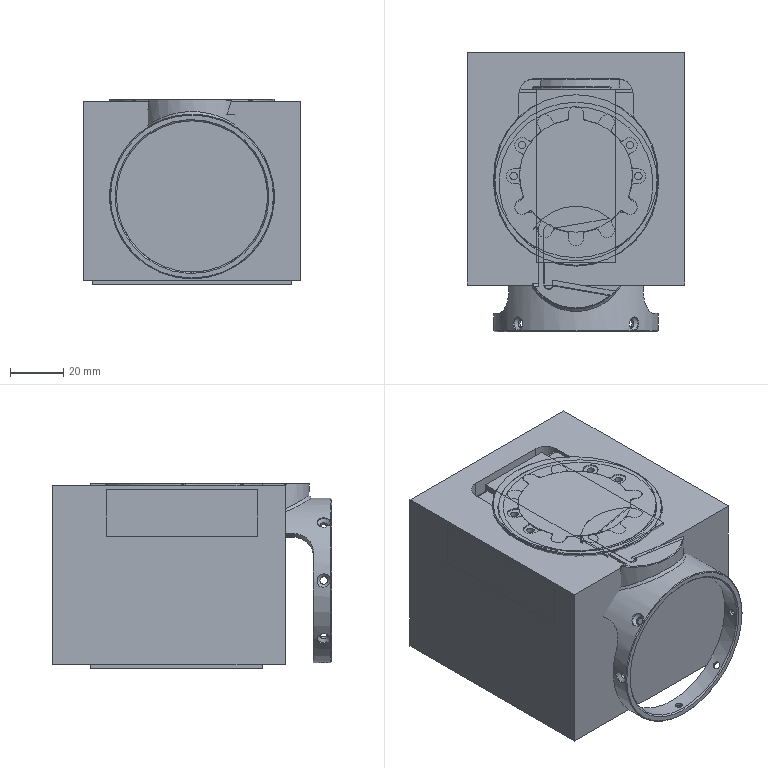NC program | NX | posted with a generic post | part box 82 x 105.2 x 70 mm
Lines 21226 to 22991 of 123648, first 1627 of 1738 lines:
(中心钻 , TOOL : 倒角刀D4)
N42414 T11 M6
N42416 G53
N42418 G19 G0 G90 Y31.15 Z-35. S2600 M3
N42420 G43 X-72.5 H11
N42422 G94 G81 G98 X-13.2 F200. R-15.
N42424 Y30.85 Z-31.5
N42426 Y31.15 Z-28.
N42428 Y30.85 Z-24.5
N42430 Y31.15 Z-21.
N42432 G80
(中心钻_COPY , TOOL : 倒角刀D4)
N42434 G17 G0 X-55. Y43.301
N42436 Z-28.
N42438 G81 X-23.135 Y16.562 F200. R-28.
N42440 G80
N42442 G0 X-53.52 Y45.117 Z-28.
N42444 X-51.98 Y46.883
N42446 X-50.382 Y48.597
N42448 X-48.727 Y50.256
N42450 X-47.018 Y51.859
N42452 X-45.256 Y53.403
N42454 X-43.443 Y54.888
N42456 X-41.582 Y56.311
N42458 X-39.673 Y57.672
N42460 X-37.721 Y58.967
N42462 X-35.726 Y60.197
N42464 X-33.691 Y61.359
N42466 X-31.619 Y62.452
N42468 X-29.511 Y63.475
N42470 X-27.37 Y64.427
N42472 X-25.198 Y65.307
N42474 X-22.998 Y66.114
N42476 X-20.772 Y66.847
N42478 X-18.523 Y67.505
N42480 X-16.254 Y68.087
N42482 X-13.966 Y68.593
N42484 X-11.662 Y69.022
N42486 X-9.345 Y69.373
N42488 X-7.018 Y69.647
N42490 X-4.683 Y69.843
N42492 X-2.343 Y69.961
N42494 G18 X0. Y70.
N42496 G17 X2.343 Y69.961
N42498 X4.683 Y69.843
N42500 X7.018 Y69.647
N42502 X9.345 Y69.373
N42504 X11.662 Y69.022
N42506 X13.966 Y68.593
N42508 X16.254 Y68.087
N42510 X18.523 Y67.505
N42512 X20.772 Y66.847
N42514 X22.998 Y66.114
N42516 X25.198 Y65.307
N42518 X27.37 Y64.427
N42520 X29.511 Y63.475
N42522 X31.619 Y62.452
N42524 X33.691 Y61.359
N42526 X35.726 Y60.197
N42528 X37.721 Y58.967
N42530 X39.673 Y57.672
N42532 X41.582 Y56.311
N42534 X43.443 Y54.888
N42536 X45.256 Y53.403
N42538 X47.018 Y51.859
N42540 X48.727 Y50.256
N42542 X50.382 Y48.597
N42544 X51.98 Y46.883
N42546 X53.52 Y45.117
N42548 X55. Y43.301
N42550 G81 X23.135 Y16.562 F200. R-28.
N42552 G80
(中心钻_COPY_COPY , TOOL : 倒角刀D4)
N42554 G0 Z-3.
N42556 X-50.902 Y48.052
N42558 G81 X-21.355 Y18.505 F200. R-3.
N42560 G80
N42562 G0 X-52.47 Y46.335 Z-3.
N42564 X-53.98 Y44.566
N42566 X-55.431 Y42.749
N42568 X-56.82 Y40.884
N42570 X-58.147 Y38.974
N42572 X-59.409 Y37.021
N42574 X-60.606 Y35.027
N42576 X-61.736 Y32.995
N42578 X-62.798 Y30.926
N42580 X-63.79 Y28.823
N42582 X-64.713 Y26.688
N42584 X-65.563 Y24.524
N42586 X-66.342 Y22.333
N42588 X-67.047 Y20.117
N42590 X-67.678 Y17.879
N42592 X-68.235 Y15.621
N42594 X-68.716 Y13.346
N42596 X-69.121 Y11.056
N42598 X-69.45 Y8.754
N42600 X-69.703 Y6.442
N42602 X-69.878 Y4.123
N42604 X-69.977 Y1.8
N42606 X-69.998 Y-0.525
N42608 G19 X-69.942 Y-2.85
N42610 G81 X-30.2 F200. R-32.
N42612 G80
N42614 G17 G0 X-69.807 Y-5.2 Z-3.
N42616 X-69.592 Y-7.544
N42618 X-69.299 Y-9.88
N42620 X-68.928 Y-12.204
N42622 X-68.479 Y-14.515
N42624 X-67.952 Y-16.809
N42626 X-67.348 Y-19.084
N42628 X-66.669 Y-21.338
N42630 X-65.913 Y-23.567
N42632 X-65.084 Y-25.77
N42634 X-64.18 Y-27.944
N42636 X-63.205 Y-30.086
N42638 X-62.157 Y-32.194
N42640 X-61.04 Y-34.266
N42642 X-59.853 Y-36.299
N42644 X-58.599 Y-38.291
N42646 X-57.278 Y-40.239
N42648 X-55.893 Y-42.142
N42650 X-54.444 Y-43.998
N42652 X-52.934 Y-45.804
N42654 X-51.364 Y-47.557
N42656 X-49.736 Y-49.258
N42658 X-48.052 Y-50.902
N42660 G81 X-21.355 Y-24.205 F200. R-3.
N42662 G80
N42664 G0 X-46.352 Y-52.455 Z-3.
N42666 X-44.601 Y-53.951
N42668 X-42.803 Y-55.389
N42670 X-40.958 Y-56.767
N42672 X-39.069 Y-58.083
N42674 X-37.137 Y-59.336
N42676 X-35.166 Y-60.526
N42678 X-33.156 Y-61.65
N42680 X-31.11 Y-62.707
N42682 X-29.031 Y-63.696
N42684 X-26.92 Y-64.616
N42686 X-24.781 Y-65.467
N42688 X-22.614 Y-66.247
N42690 X-20.423 Y-66.954
N42692 X-18.21 Y-67.59
N42694 X-15.977 Y-68.152
N42696 X-13.727 Y-68.641
N42698 X-11.462 Y-69.055
N42700 X-9.184 Y-69.395
N42702 X-6.897 Y-69.659
N42704 X-4.602 Y-69.849
N42706 X-2.302 Y-69.962
N42708 G18 X0. Y-70.
N42710 G81 Y-33.05 F200. R-34.85
N42712 G80
N42714 G17 G0 X2.302 Y-69.962 Z-3.
N42716 X4.602 Y-69.849
N42718 X6.897 Y-69.659
N42720 X9.184 Y-69.395
N42722 X11.462 Y-69.055
N42724 X13.727 Y-68.641
N42726 X15.977 Y-68.152
N42728 X18.21 Y-67.59
N42730 X20.423 Y-66.954
N42732 X22.614 Y-66.247
N42734 X24.781 Y-65.467
N42736 X26.92 Y-64.616
N42738 X29.031 Y-63.696
N42740 X31.11 Y-62.707
N42742 X33.156 Y-61.65
N42744 X35.166 Y-60.526
N42746 X37.137 Y-59.336
N42748 X39.069 Y-58.083
N42750 X40.958 Y-56.767
N42752 X42.803 Y-55.389
N42754 X44.601 Y-53.951
N42756 X46.352 Y-52.455
N42758 X48.052 Y-50.902
N42760 G81 X21.355 Y-24.205 F200. R-3.
N42762 G80
N42764 G0 X49.736 Y-49.258 Z-3.
N42766 X51.364 Y-47.557
N42768 X52.934 Y-45.804
N42770 X54.444 Y-43.998
N42772 X55.893 Y-42.142
N42774 X57.278 Y-40.239
N42776 X58.599 Y-38.291
N42778 X59.853 Y-36.299
N42780 X61.04 Y-34.266
N42782 X62.157 Y-32.194
N42784 X63.205 Y-30.086
N42786 X64.18 Y-27.944
N42788 X65.084 Y-25.77
N42790 X65.913 Y-23.567
N42792 X66.669 Y-21.338
N42794 X67.348 Y-19.084
N42796 X67.952 Y-16.809
N42798 X68.479 Y-14.515
N42800 X68.928 Y-12.204
N42802 X69.299 Y-9.88
N42804 X69.592 Y-7.544
N42806 X69.807 Y-5.2
N42808 G19 X69.942 Y-2.85
N42810 G81 X30.2 F200. R32.
N42812 G80
N42814 G17 G0 X69.998 Y-0.525 Z-3.
N42816 X69.977 Y1.8
N42818 X69.878 Y4.123
N42820 X69.703 Y6.442
N42822 X69.45 Y8.754
N42824 X69.121 Y11.056
N42826 X68.716 Y13.346
N42828 X68.235 Y15.621
N42830 X67.678 Y17.879
N42832 X67.047 Y20.117
N42834 X66.342 Y22.333
N42836 X65.563 Y24.524
N42838 X64.713 Y26.688
N42840 X63.79 Y28.823
N42842 X62.798 Y30.926
N42844 X61.736 Y32.995
N42846 X60.606 Y35.027
N42848 X59.409 Y37.021
N42850 X58.147 Y38.974
N42852 X56.82 Y40.884
N42854 X55.431 Y42.749
N42856 X53.98 Y44.566
N42858 X52.47 Y46.335
N42860 X50.902 Y48.052
N42862 G81 X21.355 Y18.505 F200. R-3.
N42864 G80
N42866 M5
(高版本钻孔 , TOOL : 钻头D1.7)
N42868 T17 M6
N42870 G53
N42872 G17 G0 G90 X47.336 Y36.869 S4000 M3
N42874 G43 Z-28. H17
N42876 G94 G83 G98 X20.689 Y14.51 F150. Q0.746 R-26.
N42878 G80
N42880 G0 X44.933 Y39.763 Z-28.
N42882 X42.353 Y42.5
N42884 X39.607 Y45.07
N42886 X36.706 Y47.463
N42888 X33.66 Y49.669
N42890 X30.482 Y51.68
N42892 X27.184 Y53.489
N42894 X23.779 Y55.087
N42896 X20.281 Y56.468
N42898 X16.704 Y57.628
N42900 X13.06 Y58.561
N42902 X9.366 Y59.265
N42904 X5.634 Y59.735
N42906 X1.881 Y59.971
N42908 X-1.881
N42910 X-5.634 Y59.735
N42912 X-9.366 Y59.265
N42914 X-13.06 Y58.561
N42916 X-16.704 Y57.628
N42918 X-20.281 Y56.468
N42920 X-23.779 Y55.087
N42922 X-27.184 Y53.489
N42924 X-30.482 Y51.68
N42926 X-33.66 Y49.669
N42928 X-36.706 Y47.463
N42930 X-39.607 Y45.07
N42932 X-42.353 Y42.5
N42934 X-44.933 Y39.763
N42936 X-47.336 Y36.869
N42938 G83 X-20.689 Y14.51 F150. Q0.746 R-26.
N42940 G80
(高版本钻孔_COPY , TOOL : 钻头D1.7)
N42942 G19 G0 Y30.85 Z-31.5
N42944 X-51.461
N42946 G83 X-10.319 F150. Q0.59 R-12.
N42948 Z-24.5
N42950 G80
N42952 M5
(高版本钻孔_COPY_COPY , TOOL : 钻头D3.2)
N42954 T16 M6
N42956 G53
N42958 G19 G0 G90 Y31.15 Z-35. S4000 M3
N42960 G43 X-51.28 H16
N42962 G94 G83 G98 X-9.839 F100. Q0.831 R-12.
N42964 Z-28.
N42966 Z-21.
N42968 G80
N42970 M5
(高版本钻孔_COPY_COPY_COPY , TOOL : 钻头D2.8)
N42972 T19 M6
N42974 G53
N42976 G17 G0 G90 X-43.827 Y40.977 S3000 M3
N42978 G43 Z-3. H19
N42980 G94 G83 G98 X-18.497 Y15.647 F100. Q1.171 R-1.
N42982 G80
N42984 G0 X-46.263 Y38.207 Z-3.
N42986 X-48.523 Y35.292
N42988 X-50.6 Y32.244
N42990 X-52.486 Y29.074
N42992 X-54.173 Y25.793
N42994 X-55.655 Y22.416
N42996 X-56.928 Y18.954
N42998 X-57.985 Y15.42
N43000 X-58.823 Y11.828
N43002 X-59.438 Y8.191
N43004 X-59.829 Y4.523
N43006 X-59.994 Y0.838
N43008 G19 X-59.932 Y-2.85
N43010 G83 X-26.159 F100. Q1.171 R-29.
N43012 G80
N43014 G17 G0 X-59.658 Y-6.4 Z-3.
N43016 X-59.173 Y-9.927
N43018 X-58.48 Y-13.419
N43020 X-57.581 Y-16.863
N43022 X-56.48 Y-20.249
N43024 X-55.18 Y-23.563
N43026 X-53.685 Y-26.794
N43028 X-52.001 Y-29.931
N43030 X-50.135 Y-32.962
N43032 X-48.091 Y-35.878
N43034 X-45.879 Y-38.667
N43036 X-43.505 Y-41.32
N43038 X-40.977 Y-43.827
N43040 G83 X-18.497 Y-21.347 F100. Q1.171 R-1.
N43042 G80
N43044 G0 X-38.153 Y-46.307 Z-3.
N43046 X-35.179 Y-48.605
N43048 X-32.067 Y-50.712
N43050 X-28.829 Y-52.62
N43052 X-25.478 Y-54.322
N43054 X-22.027 Y-55.811
N43056 X-18.489 Y-57.08
N43058 X-14.879 Y-58.126
N43060 X-11.211 Y-58.943
N43062 X-7.498 Y-59.53
N43064 X-3.757 Y-59.882
N43066 G18 X0. Y-60.
N43068 G83 Y-29.009 F100. Q1.171 R-31.85
N43070 G80
N43072 G17 G0 X3.757 Y-59.882 Z-3.
N43074 X7.498 Y-59.53
N43076 X11.211 Y-58.943
N43078 X14.879 Y-58.126
N43080 X18.489 Y-57.08
N43082 X22.027 Y-55.811
N43084 X25.478 Y-54.322
N43086 X28.829 Y-52.62
N43088 X32.067 Y-50.712
N43090 X35.179 Y-48.605
N43092 X38.153 Y-46.307
N43094 X40.977 Y-43.827
N43096 G83 X18.497 Y-21.347 F100. Q1.171 R-1.
N43098 G80
N43100 G0 X43.505 Y-41.32 Z-3.
N43102 X45.879 Y-38.667
N43104 X48.091 Y-35.878
N43106 X50.135 Y-32.962
N43108 X52.001 Y-29.931
N43110 X53.685 Y-26.794
N43112 X55.18 Y-23.563
N43114 X56.48 Y-20.249
N43116 X57.581 Y-16.863
N43118 X58.48 Y-13.419
N43120 X59.173 Y-9.927
N43122 X59.658 Y-6.4
N43124 G19 X59.932 Y-2.85
N43126 G83 X26.159 F100. Q1.171 R33.
N43128 G80
N43130 G17 G0 X59.994 Y0.838 Z-3.
N43132 X59.829 Y4.523
N43134 X59.438 Y8.191
N43136 X58.823 Y11.828
N43138 X57.985 Y15.42
N43140 X56.928 Y18.954
N43142 X55.655 Y22.416
N43144 X54.173 Y25.793
N43146 X52.486 Y29.074
N43148 X50.6 Y32.244
N43150 X48.523 Y35.292
N43152 X46.263 Y38.207
N43154 X43.827 Y40.977
N43156 G83 X18.497 Y15.647 F100. Q1.171 R-1.
N43158 G80
N43160 M5
(高版本钻孔_COPY_COPY_COPY_COPY , TOOL : 倒角刀D5)
N43162 T29 M6
N43164 G53
N43166 G17 G0 G90 X-43.827 Y40.977 S1200 M3
N43168 G43 Z-3. H29
N43170 G94 G81 G98 X-19.799 Y16.949 F40. R-1.
N43172 G80
N43174 G0 X-46.263 Y38.207 Z-3.
N43176 X-48.523 Y35.292
N43178 X-50.6 Y32.244
N43180 X-52.486 Y29.074
N43182 X-54.173 Y25.793
N43184 X-55.655 Y22.416
N43186 X-56.928 Y18.954
N43188 X-57.985 Y15.42
N43190 X-58.823 Y11.828
N43192 X-59.438 Y8.191
N43194 X-59.829 Y4.523
N43196 X-59.994 Y0.838
N43198 G19 X-59.932 Y-2.85
N43200 G81 X-28. F40. R-29.
N43202 G80
N43204 G17 G0 X-59.658 Y-6.4 Z-3.
N43206 X-59.173 Y-9.927
N43208 X-58.48 Y-13.419
N43210 X-57.581 Y-16.863
N43212 X-56.48 Y-20.249
N43214 X-55.18 Y-23.563
N43216 X-53.685 Y-26.794
N43218 X-52.001 Y-29.931
N43220 X-50.135 Y-32.962
N43222 X-48.091 Y-35.878
N43224 X-45.879 Y-38.667
N43226 X-43.505 Y-41.32
N43228 X-40.977 Y-43.827
N43230 G81 X-19.799 Y-22.649 F40. R-1.
N43232 G80
N43234 G0 X-38.153 Y-46.307 Z-3.
N43236 X-35.179 Y-48.605
N43238 X-32.067 Y-50.712
N43240 X-28.829 Y-52.62
N43242 X-25.478 Y-54.322
N43244 X-22.027 Y-55.811
N43246 X-18.489 Y-57.08
N43248 X-14.879 Y-58.126
N43250 X-11.211 Y-58.943
N43252 X-7.498 Y-59.53
N43254 X-3.757 Y-59.882
N43256 G18 X0. Y-60.
N43258 G81 Y-30.85 F40. R-31.85
N43260 G80
N43262 G17 G0 X3.757 Y-59.882 Z-3.
N43264 X7.498 Y-59.53
N43266 X11.211 Y-58.943
N43268 X14.879 Y-58.126
N43270 X18.489 Y-57.08
N43272 X22.027 Y-55.811
N43274 X25.478 Y-54.322
N43276 X28.829 Y-52.62
N43278 X32.067 Y-50.712
N43280 X35.179 Y-48.605
N43282 X38.153 Y-46.307
N43284 X40.977 Y-43.827
N43286 G81 X19.799 Y-22.649 F40. R-1.
N43288 G80
N43290 G0 X43.505 Y-41.32 Z-3.
N43292 X45.879 Y-38.667
N43294 X48.091 Y-35.878
N43296 X50.135 Y-32.962
N43298 X52.001 Y-29.931
N43300 X53.685 Y-26.794
N43302 X55.18 Y-23.563
N43304 X56.48 Y-20.249
N43306 X57.581 Y-16.863
N43308 X58.48 Y-13.419
N43310 X59.173 Y-9.927
N43312 X59.658 Y-6.4
N43314 G19 X59.932 Y-2.85
N43316 G81 X28. F40. R33.
N43318 G80
N43320 G17 G0 X59.994 Y0.838 Z-3.
N43322 X59.829 Y4.523
N43324 X59.438 Y8.191
N43326 X58.823 Y11.828
N43328 X57.985 Y15.42
N43330 X56.928 Y18.954
N43332 X55.655 Y22.416
N43334 X54.173 Y25.793
N43336 X52.486 Y29.074
N43338 X50.6 Y32.244
N43340 X48.523 Y35.292
N43342 X46.263 Y38.207
N43344 X43.827 Y40.977
N43346 G81 X19.799 Y16.949 F40. R-1.
N43348 G80
N43350 M5
(单向轮廓精光_3 , TOOL : 光刀D6)
N43352 T06 M6
N43354 G53
N43356 G19 G0 G90 Y34.151 Z-32.839 S8000 M3
N43358 G43 X-71.1 H6
N43360 X-16.508
N43362 G41 G94 G1 Y34.096 Z-33.955 F700. D6
N43364 G2 Y33.049 Z-34.905 R1.
N43366 G1 Y32.85 Z-34.9
N43368 Y31.25
N43370 Z-33.101
N43372 G2 Y32.25 Z-32.101 R1.
N43374 G1 Y33.21
N43376 G40
N43378 Y33.41
N43380 G0 X-16.017 Y34.151 Z-32.839
N43382 G41 G1 Y34.096 Z-33.955
N43384 G2 Y33.049 Z-34.905 R1.
N43386 G1 Y32.85 Z-34.9
N43388 Y31.25
N43390 Z-33.101
N43392 G2 Y32.25 Z-32.101 R1.
N43394 G1 Y33.21
N43396 G40
N43398 Y33.41
N43400 G0 X-15.525 Y34.151 Z-32.839
N43402 G41 G1 Y34.096 Z-33.955
N43404 G2 Y33.049 Z-34.905 R1.
N43406 G1 Y32.85 Z-34.9
N43408 Y31.25
N43410 Z-33.101
N43412 G2 Y32.25 Z-32.101 R1.
N43414 G1 Y33.21
N43416 G40
N43418 Y33.41
N43420 G0 X-15.033 Y34.151 Z-32.839
N43422 G41 G1 Y34.096 Z-33.955
N43424 G2 Y33.049 Z-34.905 R1.
N43426 G1 Y32.85 Z-34.9
N43428 Y31.25
N43430 Z-33.101
N43432 G2 Y32.25 Z-32.101 R1.
N43434 G1 Y33.21
N43436 G40
N43438 Y33.41
N43440 G0 X-14.542 Y34.151 Z-32.839
N43442 G41 G1 Y34.096 Z-33.955
N43444 G2 Y33.049 Z-34.905 R1.
N43446 G1 Y32.85 Z-34.9
N43448 Y31.25
N43450 Z-33.101
N43452 G2 Y32.25 Z-32.101 R1.
N43454 G1 Y33.21
N43456 G40
N43458 Y33.41
N43460 G0 X-14.05 Y34.151 Z-32.839
N43462 G41 G1 Y34.096 Z-33.955
N43464 G2 Y33.049 Z-34.905 R1.
N43466 G1 Y32.85 Z-34.9
N43468 Y31.25
N43470 Z-33.101
N43472 G2 Y32.25 Z-32.101 R1.
N43474 G1 Y33.21
N43476 G40
N43478 Y33.41
N43480 G0 X-71.1
N43482 Z-23.899
N43484 X-16.508
N43486 G41 G1 Y32.25
N43488 G2 Y31.25 Z-22.899 R1.
N43490 G1 Z-21.1
N43492 Y32.85
N43494 Y33.049 Z-21.095
N43496 G2 Y34.096 Z-22.045 R1.
N43498 G1 Y34.141 Z-22.961
N43500 G40
N43502 Y34.151 Z-23.161
N43504 G0 X-16.017 Y33.41 Z-23.899
N43506 G41 G1 Y32.25
N43508 G2 Y31.25 Z-22.899 R1.
N43510 G1 Z-21.1
N43512 Y32.85
N43514 Y33.049 Z-21.095
N43516 G2 Y34.096 Z-22.045 R1.
N43518 G1 Y34.141 Z-22.961
N43520 G40
N43522 Y34.151 Z-23.161
N43524 G0 X-15.525 Y33.41 Z-23.899
N43526 G41 G1 Y32.25
N43528 G2 Y31.25 Z-22.899 R1.
N43530 G1 Z-21.1
N43532 Y32.85
N43534 Y33.049 Z-21.095
N43536 G2 Y34.096 Z-22.045 R1.
N43538 G1 Y34.141 Z-22.961
N43540 G40
N43542 Y34.151 Z-23.161
N43544 G0 X-15.033 Y33.41 Z-23.899
N43546 G41 G1 Y32.25
N43548 G2 Y31.25 Z-22.899 R1.
N43550 G1 Z-21.1
N43552 Y32.85
N43554 Y33.049 Z-21.095
N43556 G2 Y34.096 Z-22.045 R1.
N43558 G1 Y34.141 Z-22.961
N43560 G40
N43562 Y34.151 Z-23.161
N43564 G0 X-14.542 Y33.41 Z-23.899
N43566 G41 G1 Y32.25
N43568 G2 Y31.25 Z-22.899 R1.
N43570 G1 Z-21.1
N43572 Y32.85
N43574 Y33.049 Z-21.095
N43576 G2 Y34.096 Z-22.045 R1.
N43578 G1 Y34.141 Z-22.961
N43580 G40
N43582 Y34.151 Z-23.161
N43584 G0 X-14.05 Y33.41 Z-23.899
N43586 G41 G1 Y32.25
N43588 G2 Y31.25 Z-22.899 R1.
N43590 G1 Z-21.1
N43592 Y32.85
N43594 Y33.049 Z-21.095
N43596 G2 Y34.096 Z-22.045 R1.
N43598 G1 Y34.141 Z-22.961
N43600 G40
N43602 Y34.151 Z-23.161
N43604 G0 X-71.1
(单向轮廓精光_3_COPY , TOOL : 光刀D6)
N43606 X-71.
N43608 Y38.87 Z-40.
N43610 X-17.
N43612 G1 X-14.
N43614 G41 Y37.87
N43616 G2 Y36.87 Z-39. R1.
N43618 G3 Y32.85 Z-34.98 R4.02
N43620 G1 Y31.17
N43622 Z-21.02
N43624 Y32.85
N43626 G3 Y36.87 Z-17. R4.02
N43628 G2 Y37.87 Z-16. R1.
N43630 G1 Y38.67
N43632 G40
N43634 Y38.87
N43636 X-17.
N43638 G0 X-71.
N43640 Z-40.
N43642 X-17.
N43644 G1 X-14.
N43646 G41 Y37.85
N43648 G2 Y36.85 Z-39. R1.
N43650 G3 Y32.85 Z-35. R4.
N43652 G1 Y31.15
N43654 Z-21.
N43656 Y32.85
N43658 G3 Y36.85 Z-17. R4.
N43660 G2 Y37.85 Z-16. R1.
N43662 G1 Y38.67
N43664 G40
N43666 Y38.87
N43668 X-17.
N43670 G0 X-71.
(单向轮廓精光_3_COPY_1 , TOOL : 光刀D6)
N43672 G18 Y73.95
N43674 X-4.218 Z-32.219
N43676 Y33.379
N43678 G41 G1 X-4.419 Z-33.361
N43680 G3 X-5.578 Z-34.172 R1.
N43682 G1 X-8.262 Z-33.699
N43684 G2 X-8.7 Z-33.653 R3.1
N43686 G1 Z-30.451
N43688 G3 X-7.7 Z-29.451 R1.
N43690 G1 X-6.74
N43692 G40
N43694 X-6.54
N43696 G0 X-4.218 Y32.908 Z-32.219
N43698 G41 G1 X-4.419 Z-33.361
N43700 G3 X-5.578 Z-34.172 R1.
N43702 G1 X-8.262 Z-33.699
N43704 G2 X-8.7 Z-33.653 R3.1
N43706 G1 Z-30.451
N43708 G3 X-7.7 Z-29.451 R1.
N43710 G1 X-6.74
N43712 G40
N43714 X-6.54
N43716 G0 X-4.218 Y32.438 Z-32.219
N43718 G41 G1 X-4.419 Z-33.361
N43720 G3 X-5.578 Z-34.172 R1.
N43722 G1 X-8.262 Z-33.699
N43724 G2 X-8.7 Z-33.653 R3.1
N43726 G1 Z-30.451
N43728 G3 X-7.7 Z-29.451 R1.
N43730 G1 X-6.74
N43732 G40
N43734 X-6.54
N43736 G0 X-4.218 Y31.967 Z-32.219
N43738 G41 G1 X-4.419 Z-33.361
N43740 G3 X-5.578 Z-34.172 R1.
N43742 G1 X-8.262 Z-33.699
N43744 G2 X-8.7 Z-33.653 R3.1
N43746 G1 Z-30.451
N43748 G3 X-7.7 Z-29.451 R1.
N43750 G1 X-6.74
N43752 G40
N43754 X-6.54
N43756 G0 X-4.218 Y31.496 Z-32.219
N43758 G41 G1 X-4.419 Z-33.361
N43760 G3 X-5.578 Z-34.172 R1.
N43762 G1 X-8.262 Z-33.699
N43764 G2 X-8.7 Z-33.653 R3.1
N43766 G1 Z-30.451
N43768 G3 X-7.7 Z-29.451 R1.
N43770 G1 X-6.74
N43772 G40
N43774 X-6.54
N43776 G0 X-4.218 Y31.025 Z-32.219
N43778 G41 G1 X-4.419 Z-33.361
N43780 G3 X-5.578 Z-34.172 R1.
N43782 G1 X-8.262 Z-33.699
N43784 G2 X-8.7 Z-33.653 R3.1
N43786 G1 Z-30.451
N43788 G3 X-7.7 Z-29.451 R1.
N43790 G1 X-6.74
N43792 G40
N43794 X-6.54
N43796 G0 X-4.218 Y30.554 Z-32.219
N43798 G41 G1 X-4.419 Z-33.361
N43800 G3 X-5.578 Z-34.172 R1.
N43802 G1 X-8.262 Z-33.699
N43804 G2 X-8.7 Z-33.653 R3.1
N43806 G1 Z-30.451
N43808 G3 X-7.7 Z-29.451 R1.
N43810 G1 X-6.74
N43812 G40
N43814 X-6.54
N43816 G0 X-4.218 Y30.083 Z-32.219
N43818 G41 G1 X-4.419 Z-33.361
N43820 G3 X-5.578 Z-34.172 R1.
N43822 G1 X-8.262 Z-33.699
N43824 G2 X-8.7 Z-33.653 R3.1
N43826 G1 Z-30.451
N43828 G3 X-7.7 Z-29.451 R1.
N43830 G1 X-6.74
N43832 G40
N43834 X-6.54
N43836 G0 X-4.218 Y29.613 Z-32.219
N43838 G41 G1 X-4.419 Z-33.361
N43840 G3 X-5.578 Z-34.172 R1.
N43842 G1 X-8.262 Z-33.699
N43844 G2 X-8.7 Z-33.653 R3.1
N43846 G1 Z-30.451
N43848 G3 X-7.7 Z-29.451 R1.
N43850 G1 X-6.74
N43852 G40
N43854 X-6.54
N43856 G0 X-4.218 Y29.142 Z-32.219
N43858 G41 G1 X-4.419 Z-33.361
N43860 G3 X-5.578 Z-34.172 R1.
N43862 G1 X-8.262 Z-33.699
N43864 G2 X-8.7 Z-33.653 R3.1
N43866 G1 Z-30.451
N43868 G3 X-7.7 Z-29.451 R1.
N43870 G1 X-6.74
N43872 G40
N43874 X-6.54
N43876 G0 X-4.218 Y28.671 Z-32.219
N43878 G41 G1 X-4.419 Z-33.361
N43880 G3 X-5.578 Z-34.172 R1.
N43882 G1 X-8.262 Z-33.699
N43884 G2 X-8.7 Z-33.653 R3.1
N43886 G1 Z-30.451
N43888 G3 X-7.7 Z-29.451 R1.
N43890 G1 X-6.74
N43892 G40
N43894 X-6.54
N43896 G0 X-4.218 Y28.2 Z-32.219
N43898 G41 G1 X-4.419 Z-33.361
N43900 G3 X-5.578 Z-34.172 R1.
N43902 G1 X-8.262 Z-33.699
N43904 G2 X-8.7 Z-33.653 R3.1
N43906 G1 Z-30.451
N43908 G3 X-7.7 Z-29.451 R1.
N43910 G1 X-6.74
N43912 G40
N43914 X-6.54
N43916 G0 Y73.95
N43918 Z-26.549
N43920 Y33.379
N43922 G41 G1 X-7.7
N43924 G3 X-8.7 Z-25.549 R1.
N43926 G1 Z-22.347
N43928 G2 X-8.262 Z-22.301 R3.1
N43930 G1 X-5.578 Z-21.828
N43932 G3 X-4.419 Z-22.639 R1.
N43934 G1 X-4.253 Z-23.584
N43936 G40
N43938 X-4.218 Z-23.781
N43940 G0 X-6.54 Y32.908 Z-26.549
N43942 G41 G1 X-7.7
N43944 G3 X-8.7 Z-25.549 R1.
N43946 G1 Z-22.347
N43948 G2 X-8.262 Z-22.301 R3.1
N43950 G1 X-5.578 Z-21.828
N43952 G3 X-4.419 Z-22.639 R1.
N43954 G1 X-4.253 Z-23.584
N43956 G40
N43958 X-4.218 Z-23.781
N43960 G0 X-6.54 Y32.438 Z-26.549
N43962 G41 G1 X-7.7
N43964 G3 X-8.7 Z-25.549 R1.
N43966 G1 Z-22.347
N43968 G2 X-8.262 Z-22.301 R3.1
N43970 G1 X-5.578 Z-21.828
N43972 G3 X-4.419 Z-22.639 R1.
N43974 G1 X-4.253 Z-23.584
N43976 G40
N43978 X-4.218 Z-23.781
N43980 G0 X-6.54 Y31.967 Z-26.549
N43982 G41 G1 X-7.7
N43984 G3 X-8.7 Z-25.549 R1.
N43986 G1 Z-22.347
N43988 G2 X-8.262 Z-22.301 R3.1
N43990 G1 X-5.578 Z-21.828
N43992 G3 X-4.419 Z-22.639 R1.
N43994 G1 X-4.253 Z-23.584
N43996 G40
N43998 X-4.218 Z-23.781
N44000 G0 X-6.54 Y31.496 Z-26.549
N44002 G41 G1 X-7.7
N44004 G3 X-8.7 Z-25.549 R1.
N44006 G1 Z-22.347
N44008 G2 X-8.262 Z-22.301 R3.1
N44010 G1 X-5.578 Z-21.828
N44012 G3 X-4.419 Z-22.639 R1.
N44014 G1 X-4.253 Z-23.584
N44016 G40
N44018 X-4.218 Z-23.781
N44020 G0 X-6.54 Y31.025 Z-26.549
N44022 G41 G1 X-7.7
N44024 G3 X-8.7 Z-25.549 R1.
N44026 G1 Z-22.347
N44028 G2 X-8.262 Z-22.301 R3.1
N44030 G1 X-5.578 Z-21.828
N44032 G3 X-4.419 Z-22.639 R1.
N44034 G1 X-4.253 Z-23.584
N44036 G40
N44038 X-4.218 Z-23.781
N44040 G0 X-6.54 Y30.554 Z-26.549
N44042 G41 G1 X-7.7
N44044 G3 X-8.7 Z-25.549 R1.
N44046 G1 Z-22.347
N44048 G2 X-8.262 Z-22.301 R3.1
N44050 G1 X-5.578 Z-21.828
N44052 G3 X-4.419 Z-22.639 R1.
N44054 G1 X-4.253 Z-23.584
N44056 G40
N44058 X-4.218 Z-23.781
N44060 G0 X-6.54 Y30.083 Z-26.549
N44062 G41 G1 X-7.7
N44064 G3 X-8.7 Z-25.549 R1.
N44066 G1 Z-22.347
N44068 G2 X-8.262 Z-22.301 R3.1
N44070 G1 X-5.578 Z-21.828
N44072 G3 X-4.419 Z-22.639 R1.
N44074 G1 X-4.253 Z-23.584
N44076 G40
N44078 X-4.218 Z-23.781
N44080 G0 X-6.54 Y29.613 Z-26.549
N44082 G41 G1 X-7.7
N44084 G3 X-8.7 Z-25.549 R1.
N44086 G1 Z-22.347
N44088 G2 X-8.262 Z-22.301 R3.1
N44090 G1 X-5.578 Z-21.828
N44092 G3 X-4.419 Z-22.639 R1.
N44094 G1 X-4.253 Z-23.584
N44096 G40
N44098 X-4.218 Z-23.781
N44100 G0 X-6.54 Y29.142 Z-26.549
N44102 G41 G1 X-7.7
N44104 G3 X-8.7 Z-25.549 R1.
N44106 G1 Z-22.347
N44108 G2 X-8.262 Z-22.301 R3.1
N44110 G1 X-5.578 Z-21.828
N44112 G3 X-4.419 Z-22.639 R1.
N44114 G1 X-4.253 Z-23.584
N44116 G40
N44118 X-4.218 Z-23.781
N44120 G0 X-6.54 Y28.671 Z-26.549
N44122 G41 G1 X-7.7
N44124 G3 X-8.7 Z-25.549 R1.
N44126 G1 Z-22.347
N44128 G2 X-8.262 Z-22.301 R3.1
N44130 G1 X-5.578 Z-21.828
N44132 G3 X-4.419 Z-22.639 R1.
N44134 G1 X-4.253 Z-23.584
N44136 G40
N44138 X-4.218 Z-23.781
N44140 G0 X-6.54 Y28.2 Z-26.549
N44142 G41 G1 X-7.7
N44144 G3 X-8.7 Z-25.549 R1.
N44146 G1 Z-22.347
N44148 G2 X-8.262 Z-22.301 R3.1
N44150 G1 X-5.578 Z-21.828
N44152 G3 X-4.419 Z-22.639 R1.
N44154 G1 X-4.253 Z-23.584
N44156 G40
N44158 X-4.218 Z-23.781
N44160 G0 Y73.95
(单向轮廓精光_3_COPY_1_COPY_COPY_COPY_COPY_COPY , TOOL : 光刀D6)
N44162 X16.268 Z-48.555 S7000
N44164 Y73.92
N44166 Y28.2
N44168 G41 G1 Z-42.355 F1200.
N44170 Z-40.63
N44172 G2 X13.731 Z-37.607 R3.07
N44174 G1 X-7.971 Z-33.78
N44176 G2 X-8.73 Z-33.742 R3.07
N44178 G1 Z-22.244
N44180 G2 X-7.918 Z-22.21 R3.07
N44182 G1 X13.48 Z-18.437
N44184 G2 X14.988 Z-17.707 R3.07
N44186 G1 X15.105 Z-17.603
N44188 G2 X15.676 Z-16.922 R3.07
N44190 G1 X15.811 Z-16.704
N44192 G2 X16.268 Z-15.092 R3.07
N44194 G1 Z-13.645
N44196 Z-7.645
N44198 G40
N44200 Z-7.445
N44202 G0 Y73.92
N44204 M5
(单向轮廓精光_3_COPY_1_COPY , TOOL : 光刀D2.5)
N44206 T14 M6
N44208 G53
N44210 G18 G0 G90 X-6.867 Z-34.99 S12000 M3
N44212 G43 Y74.15 H14
N44214 Y34.001
N44216 G94 G3 X-7.951 Z-35.561 R1. F1500.
N44218 G1 X-8.571 Z-35.452
N44220 G2 X-10.12 Z-36.751 R1.32
N44222 G1 Z-38.5
N44224 G3 X-10.3 Z-38.68 R0.18
N44226 X-10.48 Z-38.5 R0.18
N44228 G1 Z-32.948
N44230 G3 X-9.73 Z-31.979 R1.
N44232 G0 X-6.867 Y33.853 Z-34.99
N44234 G3 X-7.951 Z-35.561 R1.
N44236 G1 X-8.571 Z-35.452
N44238 G2 X-10.12 Z-36.751 R1.32
N44240 G1 Z-38.5
N44242 G3 X-10.3 Z-38.68 R0.18
N44244 X-10.48 Z-38.5 R0.18
N44246 G1 Z-32.948
N44248 G3 X-9.73 Z-31.979 R1.
N44250 G0 X-6.867 Y33.704 Z-34.99
N44252 G3 X-7.951 Z-35.561 R1.
N44254 G1 X-8.571 Z-35.452
N44256 G2 X-10.12 Z-36.751 R1.32
N44258 G1 Z-38.5
N44260 G3 X-10.3 Z-38.68 R0.18
N44262 X-10.48 Z-38.5 R0.18
N44264 G1 Z-32.948
N44266 G3 X-9.73 Z-31.979 R1.
N44268 G0 X-6.867 Y33.555 Z-34.99
N44270 G3 X-7.951 Z-35.561 R1.
N44272 G1 X-8.571 Z-35.452
N44274 G2 X-10.12 Z-36.751 R1.32
N44276 G1 Z-38.5
N44278 G3 X-10.3 Z-38.68 R0.18
N44280 X-10.48 Z-38.5 R0.18
N44282 G1 Z-32.948
N44284 G3 X-9.73 Z-31.979 R1.
N44286 G0 X-6.867 Y33.406 Z-34.99
N44288 G3 X-7.951 Z-35.561 R1.
N44290 G1 X-8.571 Z-35.452
N44292 G2 X-10.12 Z-36.751 R1.32
N44294 G1 Z-38.5
N44296 G3 X-10.3 Z-38.68 R0.18
N44298 X-10.48 Z-38.5 R0.18
N44300 G1 Z-32.948
N44302 G3 X-9.73 Z-31.979 R1.
N44304 G0 X-6.867 Y33.258 Z-34.99
N44306 G3 X-7.951 Z-35.561 R1.
N44308 G1 X-8.571 Z-35.452
N44310 G2 X-10.12 Z-36.751 R1.32
N44312 G1 Z-38.5
N44314 G3 X-10.3 Z-38.68 R0.18
N44316 X-10.48 Z-38.5 R0.18
N44318 G1 Z-32.948
N44320 G3 X-9.73 Z-31.979 R1.
N44322 G0 X-6.867 Y33.109 Z-34.99
N44324 G3 X-7.951 Z-35.561 R1.
N44326 G1 X-8.571 Z-35.452
N44328 G2 X-10.12 Z-36.751 R1.32
N44330 G1 Z-38.5
N44332 G3 X-10.3 Z-38.68 R0.18
N44334 X-10.48 Z-38.5 R0.18
N44336 G1 Z-32.948
N44338 G3 X-9.73 Z-31.979 R1.
N44340 G0 X-6.867 Y32.96 Z-34.99
N44342 G3 X-7.951 Z-35.561 R1.
N44344 G1 X-8.571 Z-35.452
N44346 G2 X-10.12 Z-36.751 R1.32
N44348 G1 Z-38.5
N44350 G3 X-10.3 Z-38.68 R0.18
N44352 X-10.48 Z-38.5 R0.18
N44354 G1 Z-32.948
N44356 G3 X-9.73 Z-31.979 R1.
N44358 G0 X-6.867 Y32.811 Z-34.99
N44360 G3 X-7.951 Z-35.561 R1.
N44362 G1 X-8.571 Z-35.452
N44364 G2 X-10.12 Z-36.751 R1.32
N44366 G1 Z-38.5
N44368 G3 X-10.3 Z-38.68 R0.18
N44370 X-10.48 Z-38.5 R0.18
N44372 G1 Z-32.948
N44374 G3 X-9.73 Z-31.979 R1.
N44376 G0 X-6.867 Y32.663 Z-34.99
N44378 G3 X-7.951 Z-35.561 R1.
N44380 G1 X-8.571 Z-35.452
N44382 G2 X-10.12 Z-36.751 R1.32
N44384 G1 Z-38.5
N44386 G3 X-10.3 Z-38.68 R0.18
N44388 X-10.48 Z-38.5 R0.18
N44390 G1 Z-32.948
N44392 G3 X-9.73 Z-31.979 R1.
N44394 G0 X-6.867 Y32.514 Z-34.99
N44396 G3 X-7.951 Z-35.561 R1.
N44398 G1 X-8.571 Z-35.452
N44400 G2 X-10.12 Z-36.751 R1.32
N44402 G1 Z-38.5
N44404 G3 X-10.3 Z-38.68 R0.18
N44406 X-10.48 Z-38.5 R0.18
N44408 G1 Z-32.948
N44410 G3 X-9.73 Z-31.979 R1.
N44412 G0 X-6.867 Y32.365 Z-34.99
N44414 G3 X-7.951 Z-35.561 R1.
N44416 G1 X-8.571 Z-35.452
N44418 G2 X-10.12 Z-36.751 R1.32
N44420 G1 Z-38.5
N44422 G3 X-10.3 Z-38.68 R0.18
N44424 X-10.48 Z-38.5 R0.18
N44426 G1 Z-32.948
N44428 G3 X-9.73 Z-31.979 R1.
N44430 G0 X-6.867 Y32.216 Z-34.99
N44432 G3 X-7.951 Z-35.561 R1.
N44434 G1 X-8.571 Z-35.452
N44436 G2 X-10.12 Z-36.751 R1.32
N44438 G1 Z-38.5
N44440 G3 X-10.3 Z-38.68 R0.18
N44442 X-10.48 Z-38.5 R0.18
N44444 G1 Z-32.948
N44446 G3 X-9.73 Z-31.979 R1.
N44448 G0 X-6.867 Y32.068 Z-34.99
N44450 G3 X-7.951 Z-35.561 R1.
N44452 G1 X-8.571 Z-35.452
N44454 G2 X-10.12 Z-36.751 R1.32
N44456 G1 Z-38.5
N44458 G3 X-10.3 Z-38.68 R0.18
N44460 X-10.48 Z-38.5 R0.18
N44462 G1 Z-32.948
N44464 G3 X-9.73 Z-31.979 R1.
N44466 G0 X-6.867 Y31.919 Z-34.99
N44468 G3 X-7.951 Z-35.561 R1.
N44470 G1 X-8.571 Z-35.452
N44472 G2 X-10.12 Z-36.751 R1.32
N44474 G1 Z-38.5
N44476 G3 X-10.3 Z-38.68 R0.18
N44478 X-10.48 Z-38.5 R0.18
N44480 G1 Z-32.948
N44482 G3 X-9.73 Z-31.979 R1.
N44484 G0 X-6.867 Y31.77 Z-34.99
N44486 G3 X-7.951 Z-35.561 R1.
N44488 G1 X-8.571 Z-35.452
N44490 G2 X-10.12 Z-36.751 R1.32
N44492 G1 Z-38.5
N44494 G3 X-10.3 Z-38.68 R0.18
N44496 X-10.48 Z-38.5 R0.18
N44498 G1 Z-32.948
N44500 G3 X-9.73 Z-31.979 R1.
N44502 G0 X-6.867 Y31.621 Z-34.99
N44504 G3 X-7.951 Z-35.561 R1.
N44506 G1 X-8.571 Z-35.452
N44508 G2 X-10.12 Z-36.751 R1.32
N44510 G1 Z-38.5
N44512 G3 X-10.3 Z-38.68 R0.18
N44514 X-10.48 Z-38.5 R0.18
N44516 G1 Z-32.948
N44518 G3 X-9.73 Z-31.979 R1.
N44520 G0 X-6.867 Y31.473 Z-34.99
N44522 G3 X-7.951 Z-35.561 R1.
N44524 G1 X-8.571 Z-35.452
N44526 G2 X-10.12 Z-36.751 R1.32
N44528 G1 Z-38.5
N44530 G3 X-10.3 Z-38.68 R0.18
N44532 X-10.48 Z-38.5 R0.18
N44534 G1 Z-32.948
N44536 G3 X-9.73 Z-31.979 R1.
N44538 G0 X-6.867 Y31.324 Z-34.99
N44540 G3 X-7.951 Z-35.561 R1.
N44542 G1 X-8.571 Z-35.452
N44544 G2 X-10.12 Z-36.751 R1.32
N44546 G1 Z-38.5
N44548 G3 X-10.3 Z-38.68 R0.18
N44550 X-10.48 Z-38.5 R0.18
N44552 G1 Z-32.948
N44554 G3 X-9.73 Z-31.979 R1.
N44556 G0 X-6.867 Y31.175 Z-34.99
N44558 G3 X-7.951 Z-35.561 R1.
N44560 G1 X-8.571 Z-35.452
N44562 G2 X-10.12 Z-36.751 R1.32
N44564 G1 Z-38.5
N44566 G3 X-10.3 Z-38.68 R0.18
N44568 X-10.48 Z-38.5 R0.18
N44570 G1 Z-32.948
N44572 G3 X-9.73 Z-31.979 R1.
N44574 G0 X-6.867 Y31.026 Z-34.99
N44576 G3 X-7.951 Z-35.561 R1.
N44578 G1 X-8.571 Z-35.452
N44580 G2 X-10.12 Z-36.751 R1.32
N44582 G1 Z-38.5
N44584 G3 X-10.3 Z-38.68 R0.18
N44586 X-10.48 Z-38.5 R0.18
N44588 G1 Z-32.948
N44590 G3 X-9.73 Z-31.979 R1.
N44592 G0 X-6.867 Y30.878 Z-34.99
N44594 G3 X-7.951 Z-35.561 R1.
N44596 G1 X-8.571 Z-35.452
N44598 G2 X-10.12 Z-36.751 R1.32
N44600 G1 Z-38.5
N44602 G3 X-10.3 Z-38.68 R0.18
N44604 X-10.48 Z-38.5 R0.18
N44606 G1 Z-32.948
N44608 G3 X-9.73 Z-31.979 R1.
N44610 G0 X-6.867 Y30.729 Z-34.99
N44612 G3 X-7.951 Z-35.561 R1.
N44614 G1 X-8.571 Z-35.452
N44616 G2 X-10.12 Z-36.751 R1.32
N44618 G1 Z-38.5
N44620 G3 X-10.3 Z-38.68 R0.18
N44622 X-10.48 Z-38.5 R0.18
N44624 G1 Z-32.948
N44626 G3 X-9.73 Z-31.979 R1.
N44628 G0 X-6.867 Y30.58 Z-34.99
N44630 G3 X-7.951 Z-35.561 R1.
N44632 G1 X-8.571 Z-35.452
N44634 G2 X-10.12 Z-36.751 R1.32
N44636 G1 Z-38.5
N44638 G3 X-10.3 Z-38.68 R0.18
N44640 X-10.48 Z-38.5 R0.18
N44642 G1 Z-32.948
N44644 G3 X-9.73 Z-31.979 R1.
N44646 G0 X-6.867 Y30.431 Z-34.99
N44648 G3 X-7.951 Z-35.561 R1.
N44650 G1 X-8.571 Z-35.452
N44652 G2 X-10.12 Z-36.751 R1.32
N44654 G1 Z-38.5
N44656 G3 X-10.3 Z-38.68 R0.18
N44658 X-10.48 Z-38.5 R0.18
N44660 G1 Z-32.948
N44662 G3 X-9.73 Z-31.979 R1.
N44664 G0 X-6.867 Y30.283 Z-34.99
N44666 G3 X-7.951 Z-35.561 R1.
N44668 G1 X-8.571 Z-35.452
N44670 G2 X-10.12 Z-36.751 R1.32
N44672 G1 Z-38.5
N44674 G3 X-10.3 Z-38.68 R0.18
N44676 X-10.48 Z-38.5 R0.18
N44678 G1 Z-32.948
N44680 G3 X-9.73 Z-31.979 R1.
N44682 G0 X-6.867 Y30.134 Z-34.99
N44684 G3 X-7.951 Z-35.561 R1.
N44686 G1 X-8.571 Z-35.452
N44688 G2 X-10.12 Z-36.751 R1.32
N44690 G1 Z-38.5
N44692 G3 X-10.3 Z-38.68 R0.18
N44694 X-10.48 Z-38.5 R0.18
N44696 G1 Z-32.948
N44698 G3 X-9.73 Z-31.979 R1.
N44700 G0 X-6.867 Y29.985 Z-34.99
N44702 G3 X-7.951 Z-35.561 R1.
N44704 G1 X-8.571 Z-35.452
N44706 G2 X-10.12 Z-36.751 R1.32
N44708 G1 Z-38.5
N44710 G3 X-10.3 Z-38.68 R0.18
N44712 X-10.48 Z-38.5 R0.18
N44714 G1 Z-32.948
N44716 G3 X-9.73 Z-31.979 R1.
N44718 G0 X-6.867 Y29.836 Z-34.99
N44720 G3 X-7.951 Z-35.561 R1.
N44722 G1 X-8.571 Z-35.452
N44724 G2 X-10.12 Z-36.751 R1.32
N44726 G1 Z-38.5
N44728 G3 X-10.3 Z-38.68 R0.18
N44730 X-10.48 Z-38.5 R0.18
N44732 G1 Z-32.948
N44734 G3 X-9.73 Z-31.979 R1.
N44736 G0 X-6.867 Y29.688 Z-34.99
N44738 G3 X-7.951 Z-35.561 R1.
N44740 G1 X-8.571 Z-35.452
N44742 G2 X-10.12 Z-36.751 R1.32
N44744 G1 Z-38.5
N44746 G3 X-10.3 Z-38.68 R0.18
N44748 X-10.48 Z-38.5 R0.18
N44750 G1 Z-32.948
N44752 G3 X-9.73 Z-31.979 R1.
N44754 G0 X-6.867 Y29.539 Z-34.99
N44756 G3 X-7.951 Z-35.561 R1.
N44758 G1 X-8.571 Z-35.452
N44760 G2 X-10.12 Z-36.751 R1.32
N44762 G1 Z-38.5
N44764 G3 X-10.3 Z-38.68 R0.18
N44766 X-10.48 Z-38.5 R0.18
N44768 G1 Z-32.948
N44770 G3 X-9.73 Z-31.979 R1.
N44772 G0 X-6.867 Y29.39 Z-34.99
N44774 G3 X-7.951 Z-35.561 R1.
N44776 G1 X-8.571 Z-35.452
N44778 G2 X-10.12 Z-36.751 R1.32
N44780 G1 Z-38.5
N44782 G3 X-10.3 Z-38.68 R0.18
N44784 X-10.48 Z-38.5 R0.18
N44786 G1 Z-32.948
N44788 G3 X-9.73 Z-31.979 R1.
N44790 G0 X-6.867 Y29.241 Z-34.99
N44792 G3 X-7.951 Z-35.561 R1.
N44794 G1 X-8.571 Z-35.452
N44796 G2 X-10.12 Z-36.751 R1.32
N44798 G1 Z-38.5
N44800 G3 X-10.3 Z-38.68 R0.18
N44802 X-10.48 Z-38.5 R0.18
N44804 G1 Z-32.948
N44806 G3 X-9.73 Z-31.979 R1.
N44808 G0 X-6.867 Y29.093 Z-34.99
N44810 G3 X-7.951 Z-35.561 R1.
N44812 G1 X-8.571 Z-35.452
N44814 G2 X-10.12 Z-36.751 R1.32
N44816 G1 Z-38.5
N44818 G3 X-10.3 Z-38.68 R0.18
N44820 X-10.48 Z-38.5 R0.18
N44822 G1 Z-32.948
N44824 G3 X-9.73 Z-31.979 R1.
N44826 G0 X-6.867 Y28.944 Z-34.99
N44828 G3 X-7.951 Z-35.561 R1.
N44830 G1 X-8.571 Z-35.452
N44832 G2 X-10.12 Z-36.751 R1.32
N44834 G1 Z-38.5
N44836 G3 X-10.3 Z-38.68 R0.18
N44838 X-10.48 Z-38.5 R0.18
N44840 G1 Z-32.948
N44842 G3 X-9.73 Z-31.979 R1.
N44844 G0 X-6.867 Y28.795 Z-34.99
N44846 G3 X-7.951 Z-35.561 R1.
N44848 G1 X-8.571 Z-35.452
N44850 G2 X-10.12 Z-36.751 R1.32
N44852 G1 Z-38.5
N44854 G3 X-10.3 Z-38.68 R0.18
N44856 X-10.48 Z-38.5 R0.18
N44858 G1 Z-32.948
N44860 G3 X-9.73 Z-31.979 R1.
N44862 G0 X-6.867 Y28.646 Z-34.99
N44864 G3 X-7.951 Z-35.561 R1.
N44866 G1 X-8.571 Z-35.452
N44868 G2 X-10.12 Z-36.751 R1.32
N44870 G1 Z-38.5
N44872 G3 X-10.3 Z-38.68 R0.18
N44874 X-10.48 Z-38.5 R0.18
N44876 G1 Z-32.948
N44878 G3 X-9.73 Z-31.979 R1.
N44880 G0 X-6.867 Y28.498 Z-34.99
N44882 G3 X-7.951 Z-35.561 R1.
N44884 G1 X-8.571 Z-35.452
N44886 G2 X-10.12 Z-36.751 R1.32
N44888 G1 Z-38.5
N44890 G3 X-10.3 Z-38.68 R0.18
N44892 X-10.48 Z-38.5 R0.18
N44894 G1 Z-32.948
N44896 G3 X-9.73 Z-31.979 R1.
N44898 G0 X-6.867 Y28.349 Z-34.99
N44900 G3 X-7.951 Z-35.561 R1.
N44902 G1 X-8.571 Z-35.452
N44904 G2 X-10.12 Z-36.751 R1.32
N44906 G1 Z-38.5
N44908 G3 X-10.3 Z-38.68 R0.18
N44910 X-10.48 Z-38.5 R0.18
N44912 G1 Z-32.948
N44914 G3 X-9.73 Z-31.979 R1.
N44916 G0 X-6.867 Y28.2 Z-34.99
N44918 G3 X-7.951 Z-35.561 R1.
N44920 G1 X-8.571 Z-35.452
N44922 G2 X-10.12 Z-36.751 R1.32
N44924 G1 Z-38.5
N44926 G3 X-10.3 Z-38.68 R0.18
N44928 X-10.48 Z-38.5 R0.18
N44930 G1 Z-32.948
N44932 G3 X-9.73 Z-31.979 R1.
N44934 G0 Y74.15
N44936 Z-24.021
N44938 Y34.001
N44940 G3 X-10.48 Z-23.052 R1.
N44942 G1 Z-17.5
N44944 G3 X-10.3 Z-17.32 R0.18
N44946 X-10.12 Z-17.5 R0.18
N44948 G1 Z-19.249
N44950 G2 X-8.571 Z-20.548 R1.32
N44952 G1 X-7.951 Z-20.439
N44954 G3 X-6.867 Z-21.01 R1.
N44956 G0 X-9.73 Y33.853 Z-24.021
N44958 G3 X-10.48 Z-23.052 R1.
N44960 G1 Z-17.5
N44962 G3 X-10.3 Z-17.32 R0.18
N44964 X-10.12 Z-17.5 R0.18
N44966 G1 Z-19.249
N44968 G2 X-8.571 Z-20.548 R1.32
N44970 G1 X-7.951 Z-20.439
N44972 G3 X-6.867 Z-21.01 R1.
N44974 G0 X-9.73 Y33.704 Z-24.021
N44976 G3 X-10.48 Z-23.052 R1.
N44978 G1 Z-17.5
N44980 G3 X-10.3 Z-17.32 R0.18
N44982 X-10.12 Z-17.5 R0.18
N44984 G1 Z-19.249
N44986 G2 X-8.571 Z-20.548 R1.32
N44988 G1 X-7.951 Z-20.439
N44990 G3 X-6.867 Z-21.01 R1.
N44992 G0 X-9.73 Y33.555 Z-24.021
N44994 G3 X-10.48 Z-23.052 R1.
N44996 G1 Z-17.5
N44998 G3 X-10.3 Z-17.32 R0.18
N45000 X-10.12 Z-17.5 R0.18
N45002 G1 Z-19.249
N45004 G2 X-8.571 Z-20.548 R1.32
N45006 G1 X-7.951 Z-20.439
N45008 G3 X-6.867 Z-21.01 R1.
N45010 G0 X-9.73 Y33.406 Z-24.021
N45012 G3 X-10.48 Z-23.052 R1.
N45014 G1 Z-17.5
N45016 G3 X-10.3 Z-17.32 R0.18
N45018 X-10.12 Z-17.5 R0.18
N45020 G1 Z-19.249
N45022 G2 X-8.571 Z-20.548 R1.32
N45024 G1 X-7.951 Z-20.439
N45026 G3 X-6.867 Z-21.01 R1.
N45028 G0 X-9.73 Y33.258 Z-24.021
N45030 G3 X-10.48 Z-23.052 R1.
N45032 G1 Z-17.5
N45034 G3 X-10.3 Z-17.32 R0.18
N45036 X-10.12 Z-17.5 R0.18
N45038 G1 Z-19.249
N45040 G2 X-8.571 Z-20.548 R1.32
N45042 G1 X-7.951 Z-20.439
N45044 G3 X-6.867 Z-21.01 R1.
N45046 G0 X-9.73 Y33.109 Z-24.021
N45048 G3 X-10.48 Z-23.052 R1.
N45050 G1 Z-17.5
N45052 G3 X-10.3 Z-17.32 R0.18
N45054 X-10.12 Z-17.5 R0.18
N45056 G1 Z-19.249
N45058 G2 X-8.571 Z-20.548 R1.32
N45060 G1 X-7.951 Z-20.439
N45062 G3 X-6.867 Z-21.01 R1.
N45064 G0 X-9.73 Y32.96 Z-24.021
N45066 G3 X-10.48 Z-23.052 R1.
N45068 G1 Z-17.5
N45070 G3 X-10.3 Z-17.32 R0.18
N45072 X-10.12 Z-17.5 R0.18
N45074 G1 Z-19.249
N45076 G2 X-8.571 Z-20.548 R1.32
N45078 G1 X-7.951 Z-20.439
N45080 G3 X-6.867 Z-21.01 R1.
N45082 G0 X-9.73 Y32.811 Z-24.021
N45084 G3 X-10.48 Z-23.052 R1.
N45086 G1 Z-17.5
N45088 G3 X-10.3 Z-17.32 R0.18
N45090 X-10.12 Z-17.5 R0.18
N45092 G1 Z-19.249
N45094 G2 X-8.571 Z-20.548 R1.32
N45096 G1 X-7.951 Z-20.439
N45098 G3 X-6.867 Z-21.01 R1.
N45100 G0 X-9.73 Y32.663 Z-24.021
N45102 G3 X-10.48 Z-23.052 R1.
N45104 G1 Z-17.5
N45106 G3 X-10.3 Z-17.32 R0.18
N45108 X-10.12 Z-17.5 R0.18
N45110 G1 Z-19.249
N45112 G2 X-8.571 Z-20.548 R1.32
N45114 G1 X-7.951 Z-20.439
N45116 G3 X-6.867 Z-21.01 R1.
N45118 G0 X-9.73 Y32.514 Z-24.021
N45120 G3 X-10.48 Z-23.052 R1.
N45122 G1 Z-17.5
N45124 G3 X-10.3 Z-17.32 R0.18
N45126 X-10.12 Z-17.5 R0.18
N45128 G1 Z-19.249
N45130 G2 X-8.571 Z-20.548 R1.32
N45132 G1 X-7.951 Z-20.439
N45134 G3 X-6.867 Z-21.01 R1.
N45136 G0 X-9.73 Y32.365 Z-24.021
N45138 G3 X-10.48 Z-23.052 R1.
N45140 G1 Z-17.5
N45142 G3 X-10.3 Z-17.32 R0.18
N45144 X-10.12 Z-17.5 R0.18
N45146 G1 Z-19.249
N45148 G2 X-8.571 Z-20.548 R1.32
N45150 G1 X-7.951 Z-20.439
N45152 G3 X-6.867 Z-21.01 R1.
N45154 G0 X-9.73 Y32.216 Z-24.021
N45156 G3 X-10.48 Z-23.052 R1.
N45158 G1 Z-17.5
N45160 G3 X-10.3 Z-17.32 R0.18
N45162 X-10.12 Z-17.5 R0.18
N45164 G1 Z-19.249
N45166 G2 X-8.571 Z-20.548 R1.32
N45168 G1 X-7.951 Z-20.439
N45170 G3 X-6.867 Z-21.01 R1.
N45172 G0 X-9.73 Y32.068 Z-24.021
N45174 G3 X-10.48 Z-23.052 R1.
N45176 G1 Z-17.5
N45178 G3 X-10.3 Z-17.32 R0.18
N45180 X-10.12 Z-17.5 R0.18
N45182 G1 Z-19.249
N45184 G2 X-8.571 Z-20.548 R1.32
N45186 G1 X-7.951 Z-20.439
N45188 G3 X-6.867 Z-21.01 R1.
N45190 G0 X-9.73 Y31.919 Z-24.021
N45192 G3 X-10.48 Z-23.052 R1.
N45194 G1 Z-17.5
N45196 G3 X-10.3 Z-17.32 R0.18
N45198 X-10.12 Z-17.5 R0.18
N45200 G1 Z-19.249
N45202 G2 X-8.571 Z-20.548 R1.32
N45204 G1 X-7.951 Z-20.439
N45206 G3 X-6.867 Z-21.01 R1.
N45208 G0 X-9.73 Y31.77 Z-24.021
N45210 G3 X-10.48 Z-23.052 R1.
N45212 G1 Z-17.5
N45214 G3 X-10.3 Z-17.32 R0.18
N45216 X-10.12 Z-17.5 R0.18
N45218 G1 Z-19.249
N45220 G2 X-8.571 Z-20.548 R1.32
N45222 G1 X-7.951 Z-20.439
N45224 G3 X-6.867 Z-21.01 R1.
N45226 G0 X-9.73 Y31.621 Z-24.021
N45228 G3 X-10.48 Z-23.052 R1.
N45230 G1 Z-17.5
N45232 G3 X-10.3 Z-17.32 R0.18
N45234 X-10.12 Z-17.5 R0.18
N45236 G1 Z-19.249
N45238 G2 X-8.571 Z-20.548 R1.32
N45240 G1 X-7.951 Z-20.439
N45242 G3 X-6.867 Z-21.01 R1.
N45244 G0 X-9.73 Y31.473 Z-24.021
N45246 G3 X-10.48 Z-23.052 R1.
N45248 G1 Z-17.5
N45250 G3 X-10.3 Z-17.32 R0.18
N45252 X-10.12 Z-17.5 R0.18
N45254 G1 Z-19.249
N45256 G2 X-8.571 Z-20.548 R1.32
N45258 G1 X-7.951 Z-20.439
N45260 G3 X-6.867 Z-21.01 R1.
N45262 G0 X-9.73 Y31.324 Z-24.021
N45264 G3 X-10.48 Z-23.052 R1.
N45266 G1 Z-17.5
N45268 G3 X-10.3 Z-17.32 R0.18
N45270 X-10.12 Z-17.5 R0.18
N45272 G1 Z-19.249
N45274 G2 X-8.571 Z-20.548 R1.32
N45276 G1 X-7.951 Z-20.439
N45278 G3 X-6.867 Z-21.01 R1.
N45280 G0 X-9.73 Y31.175 Z-24.021
N45282 G3 X-10.48 Z-23.052 R1.
N45284 G1 Z-17.5
N45286 G3 X-10.3 Z-17.32 R0.18
N45288 X-10.12 Z-17.5 R0.18
N45290 G1 Z-19.249
N45292 G2 X-8.571 Z-20.548 R1.32
N45294 G1 X-7.951 Z-20.439
N45296 G3 X-6.867 Z-21.01 R1.
N45298 G0 X-9.73 Y31.026 Z-24.021
N45300 G3 X-10.48 Z-23.052 R1.
N45302 G1 Z-17.5
N45304 G3 X-10.3 Z-17.32 R0.18
N45306 X-10.12 Z-17.5 R0.18
N45308 G1 Z-19.249
N45310 G2 X-8.571 Z-20.548 R1.32
N45312 G1 X-7.951 Z-20.439
N45314 G3 X-6.867 Z-21.01 R1.
N45316 G0 X-9.73 Y30.878 Z-24.021
N45318 G3 X-10.48 Z-23.052 R1.
N45320 G1 Z-17.5
N45322 G3 X-10.3 Z-17.32 R0.18
N45324 X-10.12 Z-17.5 R0.18
N45326 G1 Z-19.249
N45328 G2 X-8.571 Z-20.548 R1.32
N45330 G1 X-7.951 Z-20.439
N45332 G3 X-6.867 Z-21.01 R1.
N45334 G0 X-9.73 Y30.729 Z-24.021
N45336 G3 X-10.48 Z-23.052 R1.
N45338 G1 Z-17.5
N45340 G3 X-10.3 Z-17.32 R0.18
N45342 X-10.12 Z-17.5 R0.18
N45344 G1 Z-19.249
N45346 G2 X-8.571 Z-20.548 R1.32
N45348 G1 X-7.951 Z-20.439
N45350 G3 X-6.867 Z-21.01 R1.
N45352 G0 X-9.73 Y30.58 Z-24.021
N45354 G3 X-10.48 Z-23.052 R1.
N45356 G1 Z-17.5
N45358 G3 X-10.3 Z-17.32 R0.18
N45360 X-10.12 Z-17.5 R0.18
N45362 G1 Z-19.249
N45364 G2 X-8.571 Z-20.548 R1.32
N45366 G1 X-7.951 Z-20.439
N45368 G3 X-6.867 Z-21.01 R1.
N45370 G0 X-9.73 Y30.431 Z-24.021
N45372 G3 X-10.48 Z-23.052 R1.
N45374 G1 Z-17.5
N45376 G3 X-10.3 Z-17.32 R0.18
N45378 X-10.12 Z-17.5 R0.18
N45380 G1 Z-19.249
N45382 G2 X-8.571 Z-20.548 R1.32
N45384 G1 X-7.951 Z-20.439
N45386 G3 X-6.867 Z-21.01 R1.
N45388 G0 X-9.73 Y30.283 Z-24.021
N45390 G3 X-10.48 Z-23.052 R1.
N45392 G1 Z-17.5
N45394 G3 X-10.3 Z-17.32 R0.18
N45396 X-10.12 Z-17.5 R0.18
N45398 G1 Z-19.249
N45400 G2 X-8.571 Z-20.548 R1.32
N45402 G1 X-7.951 Z-20.439
N45404 G3 X-6.867 Z-21.01 R1.
N45406 G0 X-9.73 Y30.134 Z-24.021
N45408 G3 X-10.48 Z-23.052 R1.
N45410 G1 Z-17.5
N45412 G3 X-10.3 Z-17.32 R0.18
N45414 X-10.12 Z-17.5 R0.18
N45416 G1 Z-19.249
N45418 G2 X-8.571 Z-20.548 R1.32
N45420 G1 X-7.951 Z-20.439
N45422 G3 X-6.867 Z-21.01 R1.
N45424 G0 X-9.73 Y29.985 Z-24.021
N45426 G3 X-10.48 Z-23.052 R1.
N45428 G1 Z-17.5
N45430 G3 X-10.3 Z-17.32 R0.18
N45432 X-10.12 Z-17.5 R0.18
N45434 G1 Z-19.249
N45436 G2 X-8.571 Z-20.548 R1.32
N45438 G1 X-7.951 Z-20.439
N45440 G3 X-6.867 Z-21.01 R1.
N45442 G0 X-9.73 Y29.836 Z-24.021
N45444 G3 X-10.48 Z-23.052 R1.
N45446 G1 Z-17.5
N45448 G3 X-10.3 Z-17.32 R0.18
N45450 X-10.12 Z-17.5 R0.18
N45452 G1 Z-19.249
N45454 G2 X-8.571 Z-20.548 R1.32
N45456 G1 X-7.951 Z-20.439
N45458 G3 X-6.867 Z-21.01 R1.
N45460 G0 X-9.73 Y29.688 Z-24.021
N45462 G3 X-10.48 Z-23.052 R1.
N45464 G1 Z-17.5
N45466 G3 X-10.3 Z-17.32 R0.18
N45468 X-10.12 Z-17.5 R0.18
N45470 G1 Z-19.249
N45472 G2 X-8.571 Z-20.548 R1.32
N45474 G1 X-7.951 Z-20.439
N45476 G3 X-6.867 Z-21.01 R1.
N45478 G0 X-9.73 Y29.539 Z-24.021
N45480 G3 X-10.48 Z-23.052 R1.
N45482 G1 Z-17.5
N45484 G3 X-10.3 Z-17.32 R0.18
N45486 X-10.12 Z-17.5 R0.18
N45488 G1 Z-19.249
N45490 G2 X-8.571 Z-20.548 R1.32
N45492 G1 X-7.951 Z-20.439
N45494 G3 X-6.867 Z-21.01 R1.
N45496 G0 X-9.73 Y29.39 Z-24.021
N45498 G3 X-10.48 Z-23.052 R1.
N45500 G1 Z-17.5
N45502 G3 X-10.3 Z-17.32 R0.18
N45504 X-10.12 Z-17.5 R0.18
N45506 G1 Z-19.249
N45508 G2 X-8.571 Z-20.548 R1.32
N45510 G1 X-7.951 Z-20.439
N45512 G3 X-6.867 Z-21.01 R1.
N45514 G0 X-9.73 Y29.241 Z-24.021
N45516 G3 X-10.48 Z-23.052 R1.
N45518 G1 Z-17.5
N45520 G3 X-10.3 Z-17.32 R0.18
N45522 X-10.12 Z-17.5 R0.18
N45524 G1 Z-19.249
N45526 G2 X-8.571 Z-20.548 R1.32
N45528 G1 X-7.951 Z-20.439
N45530 G3 X-6.867 Z-21.01 R1.
N45532 G0 X-9.73 Y29.093 Z-24.021
N45534 G3 X-10.48 Z-23.052 R1.
N45536 G1 Z-17.5
N45538 G3 X-10.3 Z-17.32 R0.18
N45540 X-10.12 Z-17.5 R0.18
N45542 G1 Z-19.249
N45544 G2 X-8.571 Z-20.548 R1.32
N45546 G1 X-7.951 Z-20.439
N45548 G3 X-6.867 Z-21.01 R1.
N45550 G0 X-9.73 Y28.944 Z-24.021
N45552 G3 X-10.48 Z-23.052 R1.
N45554 G1 Z-17.5
N45556 G3 X-10.3 Z-17.32 R0.18
N45558 X-10.12 Z-17.5 R0.18
N45560 G1 Z-19.249
N45562 G2 X-8.571 Z-20.548 R1.32
N45564 G1 X-7.951 Z-20.439
N45566 G3 X-6.867 Z-21.01 R1.
N45568 G0 X-9.73 Y28.795 Z-24.021
N45570 G3 X-10.48 Z-23.052 R1.
N45572 G1 Z-17.5
N45574 G3 X-10.3 Z-17.32 R0.18
N45576 X-10.12 Z-17.5 R0.18
N45578 G1 Z-19.249
N45580 G2 X-8.571 Z-20.548 R1.32
N45582 G1 X-7.951 Z-20.439
N45584 G3 X-6.867 Z-21.01 R1.
N45586 G0 X-9.73 Y28.646 Z-24.021
N45588 G3 X-10.48 Z-23.052 R1.
N45590 G1 Z-17.5
N45592 G3 X-10.3 Z-17.32 R0.18
N45594 X-10.12 Z-17.5 R0.18
N45596 G1 Z-19.249
N45598 G2 X-8.571 Z-20.548 R1.32
N45600 G1 X-7.951 Z-20.439
N45602 G3 X-6.867 Z-21.01 R1.
N45604 G0 X-9.73 Y28.498 Z-24.021
N45606 G3 X-10.48 Z-23.052 R1.
N45608 G1 Z-17.5
N45610 G3 X-10.3 Z-17.32 R0.18
N45612 X-10.12 Z-17.5 R0.18
N45614 G1 Z-19.249
N45616 G2 X-8.571 Z-20.548 R1.32
N45618 G1 X-7.951 Z-20.439
N45620 G3 X-6.867 Z-21.01 R1.
N45622 G0 X-9.73 Y28.349 Z-24.021
N45624 G3 X-10.48 Z-23.052 R1.
N45626 G1 Z-17.5
N45628 G3 X-10.3 Z-17.32 R0.18
N45630 X-10.12 Z-17.5 R0.18
N45632 G1 Z-19.249
N45634 G2 X-8.571 Z-20.548 R1.32
N45636 G1 X-7.951 Z-20.439
N45638 G3 X-6.867 Z-21.01 R1.
N45640 G0 X-9.73 Y28.2 Z-24.021